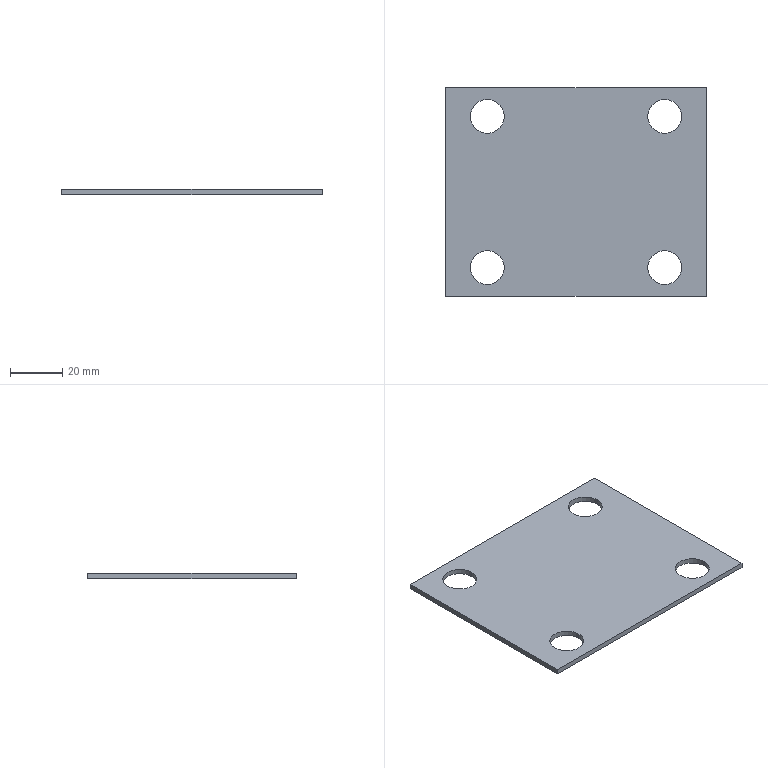Part | SolidWorks | features Extrusion 1, ICE 1 | 1 solid | 14 faces | box 100 x 80 x 2 mm | volume 14938 mm3 | cylinder 8 | plane 6 | commonest cylinder face diameters 13 x8
STEP:
#1=CARTESIAN_POINT('',(-40.5,-29.,0.));
#2=VERTEX_POINT('',#1);
#3=CARTESIAN_POINT('',(-27.5,-29.,0.));
#4=VERTEX_POINT('',#3);
#5=CARTESIAN_POINT('',(-34.,-29.,0.));
#6=DIRECTION('',(0.,0.,1.));
#7=DIRECTION('',(1.,0.,0.));
#8=AXIS2_PLACEMENT_3D('',#5,#6,#7);
#9=CIRCLE('',#8,6.5);
#10=EDGE_CURVE('',#2,#4,#9,.T.);
#11=ORIENTED_EDGE('',*,*,#10,.F.);
#12=CARTESIAN_POINT('',(-40.5,-29.,2.));
#13=VERTEX_POINT('',#12);
#14=CARTESIAN_POINT('',(-40.5,-29.,0.));
#15=DIRECTION('',(0.,0.,1.));
#16=VECTOR('',#15,1000.);
#17=LINE('',#14,#16);
#18=EDGE_CURVE('',#2,#13,#17,.T.);
#19=ORIENTED_EDGE('',*,*,#18,.T.);
#20=CARTESIAN_POINT('',(-27.5,-29.,2.));
#21=VERTEX_POINT('',#20);
#22=CARTESIAN_POINT('',(-34.,-29.,2.));
#23=DIRECTION('',(0.,0.,1.));
#24=DIRECTION('',(1.,0.,0.));
#25=AXIS2_PLACEMENT_3D('',#22,#23,#24);
#26=CIRCLE('',#25,6.5);
#27=EDGE_CURVE('',#13,#21,#26,.T.);
#28=ORIENTED_EDGE('',*,*,#27,.T.);
#29=CARTESIAN_POINT('',(-27.5,-29.,0.));
#30=DIRECTION('',(0.,0.,1.));
#31=VECTOR('',#30,1000.);
#32=LINE('',#29,#31);
#33=EDGE_CURVE('',#4,#21,#32,.T.);
#34=ORIENTED_EDGE('',*,*,#33,.F.);
#35=EDGE_LOOP('',(#11,#19,#28,#34));
#36=FACE_OUTER_BOUND('',#35,.T.);
#37=CARTESIAN_POINT('',(-34.,-29.,0.));
#38=DIRECTION('',(0.,0.,1.));
#39=DIRECTION('',(1.,0.,0.));
#40=AXIS2_PLACEMENT_3D('',#37,#38,#39);
#41=CYLINDRICAL_SURFACE('',#40,6.5);
#42=ADVANCED_FACE('',(#36),#41,.F.);
#43=CARTESIAN_POINT('',(27.5,-29.,0.));
#44=VERTEX_POINT('',#43);
#45=CARTESIAN_POINT('',(40.5,-29.,0.));
#46=VERTEX_POINT('',#45);
#47=CARTESIAN_POINT('',(34.,-29.,0.));
#48=DIRECTION('',(0.,0.,1.));
#49=DIRECTION('',(1.,0.,0.));
#50=AXIS2_PLACEMENT_3D('',#47,#48,#49);
#51=CIRCLE('',#50,6.5);
#52=EDGE_CURVE('',#44,#46,#51,.T.);
#53=ORIENTED_EDGE('',*,*,#52,.F.);
#54=CARTESIAN_POINT('',(27.5,-29.,2.));
#55=VERTEX_POINT('',#54);
#56=CARTESIAN_POINT('',(27.5,-29.,0.));
#57=DIRECTION('',(0.,0.,1.));
#58=VECTOR('',#57,1000.);
#59=LINE('',#56,#58);
#60=EDGE_CURVE('',#44,#55,#59,.T.);
#61=ORIENTED_EDGE('',*,*,#60,.T.);
#62=CARTESIAN_POINT('',(40.5,-29.,2.));
#63=VERTEX_POINT('',#62);
#64=CARTESIAN_POINT('',(34.,-29.,2.));
#65=DIRECTION('',(0.,0.,1.));
#66=DIRECTION('',(1.,0.,0.));
#67=AXIS2_PLACEMENT_3D('',#64,#65,#66);
#68=CIRCLE('',#67,6.5);
#69=EDGE_CURVE('',#55,#63,#68,.T.);
#70=ORIENTED_EDGE('',*,*,#69,.T.);
#71=CARTESIAN_POINT('',(40.5,-29.,0.));
#72=DIRECTION('',(0.,0.,1.));
#73=VECTOR('',#72,1000.);
#74=LINE('',#71,#73);
#75=EDGE_CURVE('',#46,#63,#74,.T.);
#76=ORIENTED_EDGE('',*,*,#75,.F.);
#77=EDGE_LOOP('',(#53,#61,#70,#76));
#78=FACE_OUTER_BOUND('',#77,.T.);
#79=CARTESIAN_POINT('',(34.,-29.,0.));
#80=DIRECTION('',(0.,0.,1.));
#81=DIRECTION('',(1.,0.,0.));
#82=AXIS2_PLACEMENT_3D('',#79,#80,#81);
#83=CYLINDRICAL_SURFACE('',#82,6.5);
#84=ADVANCED_FACE('',(#78),#83,.F.);
#85=CARTESIAN_POINT('',(27.5,29.,0.));
#86=VERTEX_POINT('',#85);
#87=CARTESIAN_POINT('',(40.5,29.,0.));
#88=VERTEX_POINT('',#87);
#89=CARTESIAN_POINT('',(34.,29.,0.));
#90=DIRECTION('',(0.,0.,1.));
#91=DIRECTION('',(1.,0.,0.));
#92=AXIS2_PLACEMENT_3D('',#89,#90,#91);
#93=CIRCLE('',#92,6.5);
#94=EDGE_CURVE('',#86,#88,#93,.T.);
#95=ORIENTED_EDGE('',*,*,#94,.F.);
#96=CARTESIAN_POINT('',(27.5,29.,2.));
#97=VERTEX_POINT('',#96);
#98=CARTESIAN_POINT('',(27.5,29.,0.));
#99=DIRECTION('',(0.,0.,1.));
#100=VECTOR('',#99,1000.);
#101=LINE('',#98,#100);
#102=EDGE_CURVE('',#86,#97,#101,.T.);
#103=ORIENTED_EDGE('',*,*,#102,.T.);
#104=CARTESIAN_POINT('',(40.5,29.,2.));
#105=VERTEX_POINT('',#104);
#106=CARTESIAN_POINT('',(34.,29.,2.));
#107=DIRECTION('',(0.,0.,1.));
#108=DIRECTION('',(1.,0.,0.));
#109=AXIS2_PLACEMENT_3D('',#106,#107,#108);
#110=CIRCLE('',#109,6.5);
#111=EDGE_CURVE('',#97,#105,#110,.T.);
#112=ORIENTED_EDGE('',*,*,#111,.T.);
#113=CARTESIAN_POINT('',(40.5,29.,0.));
#114=DIRECTION('',(0.,0.,1.));
#115=VECTOR('',#114,1000.);
#116=LINE('',#113,#115);
#117=EDGE_CURVE('',#88,#105,#116,.T.);
#118=ORIENTED_EDGE('',*,*,#117,.F.);
#119=EDGE_LOOP('',(#95,#103,#112,#118));
#120=FACE_OUTER_BOUND('',#119,.T.);
#121=CARTESIAN_POINT('',(34.,29.,0.));
#122=DIRECTION('',(0.,0.,1.));
#123=DIRECTION('',(1.,0.,0.));
#124=AXIS2_PLACEMENT_3D('',#121,#122,#123);
#125=CYLINDRICAL_SURFACE('',#124,6.5);
#126=ADVANCED_FACE('',(#120),#125,.F.);
#127=CARTESIAN_POINT('',(-40.5,29.,0.));
#128=VERTEX_POINT('',#127);
#129=CARTESIAN_POINT('',(-27.5,29.,0.));
#130=VERTEX_POINT('',#129);
#131=CARTESIAN_POINT('',(-34.,29.,0.));
#132=DIRECTION('',(0.,0.,1.));
#133=DIRECTION('',(1.,0.,0.));
#134=AXIS2_PLACEMENT_3D('',#131,#132,#133);
#135=CIRCLE('',#134,6.5);
#136=EDGE_CURVE('',#128,#130,#135,.T.);
#137=ORIENTED_EDGE('',*,*,#136,.F.);
#138=CARTESIAN_POINT('',(-40.5,29.,2.));
#139=VERTEX_POINT('',#138);
#140=CARTESIAN_POINT('',(-40.5,29.,0.));
#141=DIRECTION('',(0.,0.,1.));
#142=VECTOR('',#141,1000.);
#143=LINE('',#140,#142);
#144=EDGE_CURVE('',#128,#139,#143,.T.);
#145=ORIENTED_EDGE('',*,*,#144,.T.);
#146=CARTESIAN_POINT('',(-27.5,29.,2.));
#147=VERTEX_POINT('',#146);
#148=CARTESIAN_POINT('',(-34.,29.,2.));
#149=DIRECTION('',(0.,0.,1.));
#150=DIRECTION('',(1.,0.,0.));
#151=AXIS2_PLACEMENT_3D('',#148,#149,#150);
#152=CIRCLE('',#151,6.5);
#153=EDGE_CURVE('',#139,#147,#152,.T.);
#154=ORIENTED_EDGE('',*,*,#153,.T.);
#155=CARTESIAN_POINT('',(-27.5,29.,0.));
#156=DIRECTION('',(0.,0.,1.));
#157=VECTOR('',#156,1000.);
#158=LINE('',#155,#157);
#159=EDGE_CURVE('',#130,#147,#158,.T.);
#160=ORIENTED_EDGE('',*,*,#159,.F.);
#161=EDGE_LOOP('',(#137,#145,#154,#160));
#162=FACE_OUTER_BOUND('',#161,.T.);
#163=CARTESIAN_POINT('',(-34.,29.,0.));
#164=DIRECTION('',(0.,0.,1.));
#165=DIRECTION('',(1.,0.,0.));
#166=AXIS2_PLACEMENT_3D('',#163,#164,#165);
#167=CYLINDRICAL_SURFACE('',#166,6.5);
#168=ADVANCED_FACE('',(#162),#167,.F.);
#169=CARTESIAN_POINT('',(50.,-40.,0.));
#170=VERTEX_POINT('',#169);
#171=CARTESIAN_POINT('',(50.,40.,0.));
#172=VERTEX_POINT('',#171);
#173=CARTESIAN_POINT('',(50.,40.,0.));
#174=DIRECTION('',(0.,1.,0.));
#175=VECTOR('',#174,1000.);
#176=LINE('',#173,#175);
#177=EDGE_CURVE('',#170,#172,#176,.T.);
#178=ORIENTED_EDGE('',*,*,#177,.T.);
#179=CARTESIAN_POINT('',(50.,40.,2.));
#180=VERTEX_POINT('',#179);
#181=CARTESIAN_POINT('',(50.,40.,2.));
#182=DIRECTION('',(0.,0.,-1.));
#183=VECTOR('',#182,1000.);
#184=LINE('',#181,#183);
#185=EDGE_CURVE('',#180,#172,#184,.T.);
#186=ORIENTED_EDGE('',*,*,#185,.F.);
#187=CARTESIAN_POINT('',(50.,-40.,2.));
#188=VERTEX_POINT('',#187);
#189=CARTESIAN_POINT('',(50.,40.,2.));
#190=DIRECTION('',(0.,1.,0.));
#191=VECTOR('',#190,1000.);
#192=LINE('',#189,#191);
#193=EDGE_CURVE('',#188,#180,#192,.T.);
#194=ORIENTED_EDGE('',*,*,#193,.F.);
#195=CARTESIAN_POINT('',(50.,-40.,2.));
#196=DIRECTION('',(0.,0.,-1.));
#197=VECTOR('',#196,1000.);
#198=LINE('',#195,#197);
#199=EDGE_CURVE('',#188,#170,#198,.T.);
#200=ORIENTED_EDGE('',*,*,#199,.T.);
#201=EDGE_LOOP('',(#178,#186,#194,#200));
#202=FACE_OUTER_BOUND('',#201,.T.);
#203=CARTESIAN_POINT('',(50.,40.,2.));
#204=DIRECTION('',(-1.,0.,0.));
#205=DIRECTION('',(0.,0.,1.));
#206=AXIS2_PLACEMENT_3D('',#203,#204,#205);
#207=PLANE('',#206);
#208=ADVANCED_FACE('',(#202),#207,.F.);
#209=CARTESIAN_POINT('',(-50.,40.,0.));
#210=VERTEX_POINT('',#209);
#211=CARTESIAN_POINT('',(-50.,40.,0.));
#212=DIRECTION('',(-1.,0.,0.));
#213=VECTOR('',#212,1000.);
#214=LINE('',#211,#213);
#215=EDGE_CURVE('',#172,#210,#214,.T.);
#216=ORIENTED_EDGE('',*,*,#215,.T.);
#217=CARTESIAN_POINT('',(-50.,40.,2.));
#218=VERTEX_POINT('',#217);
#219=CARTESIAN_POINT('',(-50.,40.,2.));
#220=DIRECTION('',(0.,0.,-1.));
#221=VECTOR('',#220,1000.);
#222=LINE('',#219,#221);
#223=EDGE_CURVE('',#218,#210,#222,.T.);
#224=ORIENTED_EDGE('',*,*,#223,.F.);
#225=CARTESIAN_POINT('',(-50.,40.,2.));
#226=DIRECTION('',(-1.,0.,0.));
#227=VECTOR('',#226,1000.);
#228=LINE('',#225,#227);
#229=EDGE_CURVE('',#180,#218,#228,.T.);
#230=ORIENTED_EDGE('',*,*,#229,.F.);
#231=ORIENTED_EDGE('',*,*,#185,.T.);
#232=EDGE_LOOP('',(#216,#224,#230,#231));
#233=FACE_OUTER_BOUND('',#232,.T.);
#234=CARTESIAN_POINT('',(-50.,40.,2.));
#235=DIRECTION('',(0.,-1.,0.));
#236=DIRECTION('',(0.,0.,-1.));
#237=AXIS2_PLACEMENT_3D('',#234,#235,#236);
#238=PLANE('',#237);
#239=ADVANCED_FACE('',(#233),#238,.F.);
#240=CARTESIAN_POINT('',(-50.,-40.,0.));
#241=VERTEX_POINT('',#240);
#242=CARTESIAN_POINT('',(-50.,40.,0.));
#243=DIRECTION('',(0.,-1.,0.));
#244=VECTOR('',#243,1000.);
#245=LINE('',#242,#244);
#246=EDGE_CURVE('',#210,#241,#245,.T.);
#247=ORIENTED_EDGE('',*,*,#246,.T.);
#248=CARTESIAN_POINT('',(-50.,-40.,2.));
#249=VERTEX_POINT('',#248);
#250=CARTESIAN_POINT('',(-50.,-40.,2.));
#251=DIRECTION('',(0.,0.,-1.));
#252=VECTOR('',#251,1000.);
#253=LINE('',#250,#252);
#254=EDGE_CURVE('',#249,#241,#253,.T.);
#255=ORIENTED_EDGE('',*,*,#254,.F.);
#256=CARTESIAN_POINT('',(-50.,40.,2.));
#257=DIRECTION('',(0.,-1.,0.));
#258=VECTOR('',#257,1000.);
#259=LINE('',#256,#258);
#260=EDGE_CURVE('',#218,#249,#259,.T.);
#261=ORIENTED_EDGE('',*,*,#260,.F.);
#262=ORIENTED_EDGE('',*,*,#223,.T.);
#263=EDGE_LOOP('',(#247,#255,#261,#262));
#264=FACE_OUTER_BOUND('',#263,.T.);
#265=CARTESIAN_POINT('',(-50.,40.,2.));
#266=DIRECTION('',(1.,0.,0.));
#267=DIRECTION('',(0.,0.,-1.));
#268=AXIS2_PLACEMENT_3D('',#265,#266,#267);
#269=PLANE('',#268);
#270=ADVANCED_FACE('',(#264),#269,.F.);
#271=CARTESIAN_POINT('',(-50.,-40.,0.));
#272=DIRECTION('',(1.,0.,0.));
#273=VECTOR('',#272,1000.);
#274=LINE('',#271,#273);
#275=EDGE_CURVE('',#241,#170,#274,.T.);
#276=ORIENTED_EDGE('',*,*,#275,.T.);
#277=ORIENTED_EDGE('',*,*,#199,.F.);
#278=CARTESIAN_POINT('',(-50.,-40.,2.));
#279=DIRECTION('',(1.,0.,0.));
#280=VECTOR('',#279,1000.);
#281=LINE('',#278,#280);
#282=EDGE_CURVE('',#249,#188,#281,.T.);
#283=ORIENTED_EDGE('',*,*,#282,.F.);
#284=ORIENTED_EDGE('',*,*,#254,.T.);
#285=EDGE_LOOP('',(#276,#277,#283,#284));
#286=FACE_OUTER_BOUND('',#285,.T.);
#287=CARTESIAN_POINT('',(-50.,-40.,2.));
#288=DIRECTION('',(0.,1.,0.));
#289=DIRECTION('',(0.,0.,1.));
#290=AXIS2_PLACEMENT_3D('',#287,#288,#289);
#291=PLANE('',#290);
#292=ADVANCED_FACE('',(#286),#291,.F.);
#293=CARTESIAN_POINT('',(-34.,-29.,2.));
#294=DIRECTION('',(0.,0.,1.));
#295=DIRECTION('',(1.,0.,0.));
#296=AXIS2_PLACEMENT_3D('',#293,#294,#295);
#297=CIRCLE('',#296,6.5);
#298=EDGE_CURVE('',#21,#13,#297,.T.);
#299=ORIENTED_EDGE('',*,*,#298,.F.);
#300=ORIENTED_EDGE('',*,*,#27,.F.);
#301=EDGE_LOOP('',(#299,#300));
#302=FACE_BOUND('',#301,.T.);
#303=CARTESIAN_POINT('',(34.,-29.,2.));
#304=DIRECTION('',(0.,0.,1.));
#305=DIRECTION('',(1.,0.,0.));
#306=AXIS2_PLACEMENT_3D('',#303,#304,#305);
#307=CIRCLE('',#306,6.5);
#308=EDGE_CURVE('',#63,#55,#307,.T.);
#309=ORIENTED_EDGE('',*,*,#308,.F.);
#310=ORIENTED_EDGE('',*,*,#69,.F.);
#311=EDGE_LOOP('',(#309,#310));
#312=FACE_BOUND('',#311,.T.);
#313=CARTESIAN_POINT('',(34.,29.,2.));
#314=DIRECTION('',(0.,0.,1.));
#315=DIRECTION('',(1.,0.,0.));
#316=AXIS2_PLACEMENT_3D('',#313,#314,#315);
#317=CIRCLE('',#316,6.5);
#318=EDGE_CURVE('',#105,#97,#317,.T.);
#319=ORIENTED_EDGE('',*,*,#318,.F.);
#320=ORIENTED_EDGE('',*,*,#111,.F.);
#321=EDGE_LOOP('',(#319,#320));
#322=FACE_BOUND('',#321,.T.);
#323=CARTESIAN_POINT('',(-34.,29.,2.));
#324=DIRECTION('',(0.,0.,1.));
#325=DIRECTION('',(1.,0.,0.));
#326=AXIS2_PLACEMENT_3D('',#323,#324,#325);
#327=CIRCLE('',#326,6.5);
#328=EDGE_CURVE('',#147,#139,#327,.T.);
#329=ORIENTED_EDGE('',*,*,#328,.F.);
#330=ORIENTED_EDGE('',*,*,#153,.F.);
#331=EDGE_LOOP('',(#329,#330));
#332=FACE_BOUND('',#331,.T.);
#333=ORIENTED_EDGE('',*,*,#193,.T.);
#334=ORIENTED_EDGE('',*,*,#229,.T.);
#335=ORIENTED_EDGE('',*,*,#260,.T.);
#336=ORIENTED_EDGE('',*,*,#282,.T.);
#337=EDGE_LOOP('',(#333,#334,#335,#336));
#338=FACE_OUTER_BOUND('',#337,.T.);
#339=CARTESIAN_POINT('',(0.,0.,2.));
#340=DIRECTION('',(0.,0.,1.));
#341=DIRECTION('',(1.,0.,0.));
#342=AXIS2_PLACEMENT_3D('',#339,#340,#341);
#343=PLANE('',#342);
#344=ADVANCED_FACE('',(#302,#312,#322,#332,#338),#343,.T.);
#345=CARTESIAN_POINT('',(-34.,-29.,0.));
#346=DIRECTION('',(0.,0.,1.));
#347=DIRECTION('',(1.,0.,0.));
#348=AXIS2_PLACEMENT_3D('',#345,#346,#347);
#349=CIRCLE('',#348,6.5);
#350=EDGE_CURVE('',#4,#2,#349,.T.);
#351=ORIENTED_EDGE('',*,*,#350,.T.);
#352=ORIENTED_EDGE('',*,*,#10,.T.);
#353=EDGE_LOOP('',(#351,#352));
#354=FACE_BOUND('',#353,.T.);
#355=CARTESIAN_POINT('',(34.,-29.,0.));
#356=DIRECTION('',(0.,0.,1.));
#357=DIRECTION('',(1.,0.,0.));
#358=AXIS2_PLACEMENT_3D('',#355,#356,#357);
#359=CIRCLE('',#358,6.5);
#360=EDGE_CURVE('',#46,#44,#359,.T.);
#361=ORIENTED_EDGE('',*,*,#360,.T.);
#362=ORIENTED_EDGE('',*,*,#52,.T.);
#363=EDGE_LOOP('',(#361,#362));
#364=FACE_BOUND('',#363,.T.);
#365=CARTESIAN_POINT('',(34.,29.,0.));
#366=DIRECTION('',(0.,0.,1.));
#367=DIRECTION('',(1.,0.,0.));
#368=AXIS2_PLACEMENT_3D('',#365,#366,#367);
#369=CIRCLE('',#368,6.5);
#370=EDGE_CURVE('',#88,#86,#369,.T.);
#371=ORIENTED_EDGE('',*,*,#370,.T.);
#372=ORIENTED_EDGE('',*,*,#94,.T.);
#373=EDGE_LOOP('',(#371,#372));
#374=FACE_BOUND('',#373,.T.);
#375=CARTESIAN_POINT('',(-34.,29.,0.));
#376=DIRECTION('',(0.,0.,1.));
#377=DIRECTION('',(1.,0.,0.));
#378=AXIS2_PLACEMENT_3D('',#375,#376,#377);
#379=CIRCLE('',#378,6.5);
#380=EDGE_CURVE('',#130,#128,#379,.T.);
#381=ORIENTED_EDGE('',*,*,#380,.T.);
#382=ORIENTED_EDGE('',*,*,#136,.T.);
#383=EDGE_LOOP('',(#381,#382));
#384=FACE_BOUND('',#383,.T.);
#385=ORIENTED_EDGE('',*,*,#177,.F.);
#386=ORIENTED_EDGE('',*,*,#275,.F.);
#387=ORIENTED_EDGE('',*,*,#246,.F.);
#388=ORIENTED_EDGE('',*,*,#215,.F.);
#389=EDGE_LOOP('',(#385,#386,#387,#388));
#390=FACE_OUTER_BOUND('',#389,.T.);
#391=CARTESIAN_POINT('',(0.,0.,0.));
#392=DIRECTION('',(0.,0.,1.));
#393=DIRECTION('',(1.,0.,0.));
#394=AXIS2_PLACEMENT_3D('',#391,#392,#393);
#395=PLANE('',#394);
#396=ADVANCED_FACE('',(#354,#364,#374,#384,#390),#395,.F.);
#397=ORIENTED_EDGE('',*,*,#144,.F.);
#398=ORIENTED_EDGE('',*,*,#380,.F.);
#399=ORIENTED_EDGE('',*,*,#159,.T.);
#400=ORIENTED_EDGE('',*,*,#328,.T.);
#401=EDGE_LOOP('',(#397,#398,#399,#400));
#402=FACE_OUTER_BOUND('',#401,.T.);
#403=CARTESIAN_POINT('',(-34.,29.,0.));
#404=DIRECTION('',(0.,0.,1.));
#405=DIRECTION('',(1.,0.,0.));
#406=AXIS2_PLACEMENT_3D('',#403,#404,#405);
#407=CYLINDRICAL_SURFACE('',#406,6.5);
#408=ADVANCED_FACE('',(#402),#407,.F.);
#409=ORIENTED_EDGE('',*,*,#102,.F.);
#410=ORIENTED_EDGE('',*,*,#370,.F.);
#411=ORIENTED_EDGE('',*,*,#117,.T.);
#412=ORIENTED_EDGE('',*,*,#318,.T.);
#413=EDGE_LOOP('',(#409,#410,#411,#412));
#414=FACE_OUTER_BOUND('',#413,.T.);
#415=CARTESIAN_POINT('',(34.,29.,0.));
#416=DIRECTION('',(0.,0.,1.));
#417=DIRECTION('',(1.,0.,0.));
#418=AXIS2_PLACEMENT_3D('',#415,#416,#417);
#419=CYLINDRICAL_SURFACE('',#418,6.5);
#420=ADVANCED_FACE('',(#414),#419,.F.);
#421=ORIENTED_EDGE('',*,*,#60,.F.);
#422=ORIENTED_EDGE('',*,*,#360,.F.);
#423=ORIENTED_EDGE('',*,*,#75,.T.);
#424=ORIENTED_EDGE('',*,*,#308,.T.);
#425=EDGE_LOOP('',(#421,#422,#423,#424));
#426=FACE_OUTER_BOUND('',#425,.T.);
#427=CARTESIAN_POINT('',(34.,-29.,0.));
#428=DIRECTION('',(0.,0.,1.));
#429=DIRECTION('',(1.,0.,0.));
#430=AXIS2_PLACEMENT_3D('',#427,#428,#429);
#431=CYLINDRICAL_SURFACE('',#430,6.5);
#432=ADVANCED_FACE('',(#426),#431,.F.);
#433=ORIENTED_EDGE('',*,*,#18,.F.);
#434=ORIENTED_EDGE('',*,*,#350,.F.);
#435=ORIENTED_EDGE('',*,*,#33,.T.);
#436=ORIENTED_EDGE('',*,*,#298,.T.);
#437=EDGE_LOOP('',(#433,#434,#435,#436));
#438=FACE_OUTER_BOUND('',#437,.T.);
#439=CARTESIAN_POINT('',(-34.,-29.,0.));
#440=DIRECTION('',(0.,0.,1.));
#441=DIRECTION('',(1.,0.,0.));
#442=AXIS2_PLACEMENT_3D('',#439,#440,#441);
#443=CYLINDRICAL_SURFACE('',#442,6.5);
#444=ADVANCED_FACE('',(#438),#443,.F.);
#445=CLOSED_SHELL('',(#42,#84,#126,#168,#208,#239,#270,#292,#344,#396,#408,#420,#432,#444));
#446=MANIFOLD_SOLID_BREP('',#445);
#447=CARTESIAN_POINT('',(0.,0.,0.));
#448=DIRECTION('',(0.,0.,1.));
#449=DIRECTION('',(1.,0.,0.));
#450=AXIS2_PLACEMENT_3D('',#447,#448,#449);
#451=(LENGTH_UNIT()NAMED_UNIT(*)SI_UNIT(.MILLI.,.METRE.));
#452=UNCERTAINTY_MEASURE_WITH_UNIT(LENGTH_MEASURE(0.00001),#451,'','');
#453=(NAMED_UNIT(*)PLANE_ANGLE_UNIT()SI_UNIT($,.RADIAN.));
#454=(NAMED_UNIT(*)SI_UNIT($,.STERADIAN.)SOLID_ANGLE_UNIT());
#455=(GEOMETRIC_REPRESENTATION_CONTEXT(3)GLOBAL_UNCERTAINTY_ASSIGNED_CONTEXT((#452))GLOBAL_UNIT_ASSIGNED_CONTEXT((#451,#453,#454))REPRESENTATION_CONTEXT('',''));
#456=ADVANCED_BREP_SHAPE_REPRESENTATION('',(#446,#450),#455);